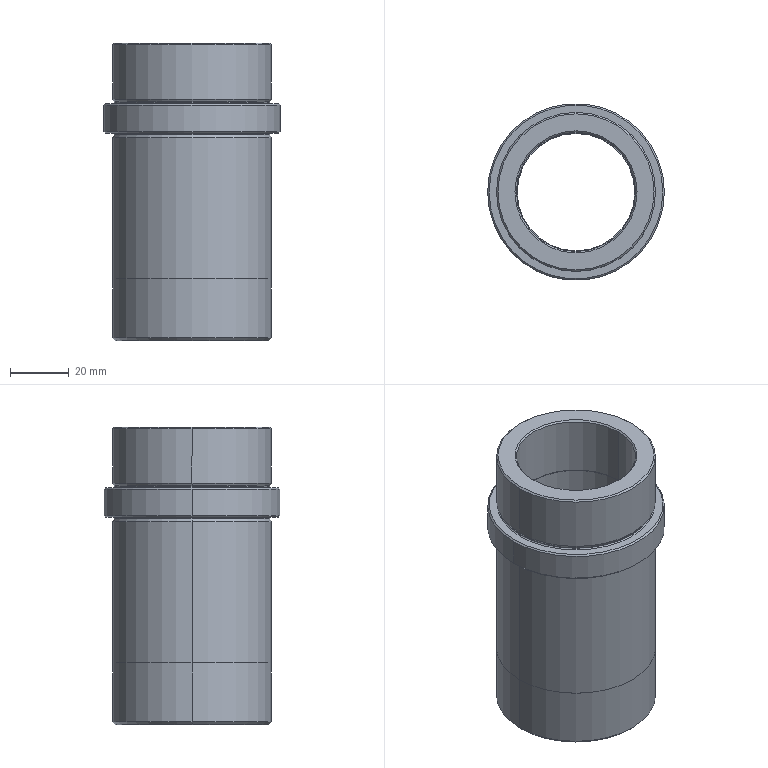Part | STEP file | Bushing BG - PN_0001 - cut | 1 solid | 42 faces | box 60 x 60 x 101 mm | volume 108263 mm3 | cone 14 | cylinder 12 | torus 10 | plane 6 | commonest cylinder face diameters 54 x4 40 x2 40.5 x2 53.98 x2 60 x2